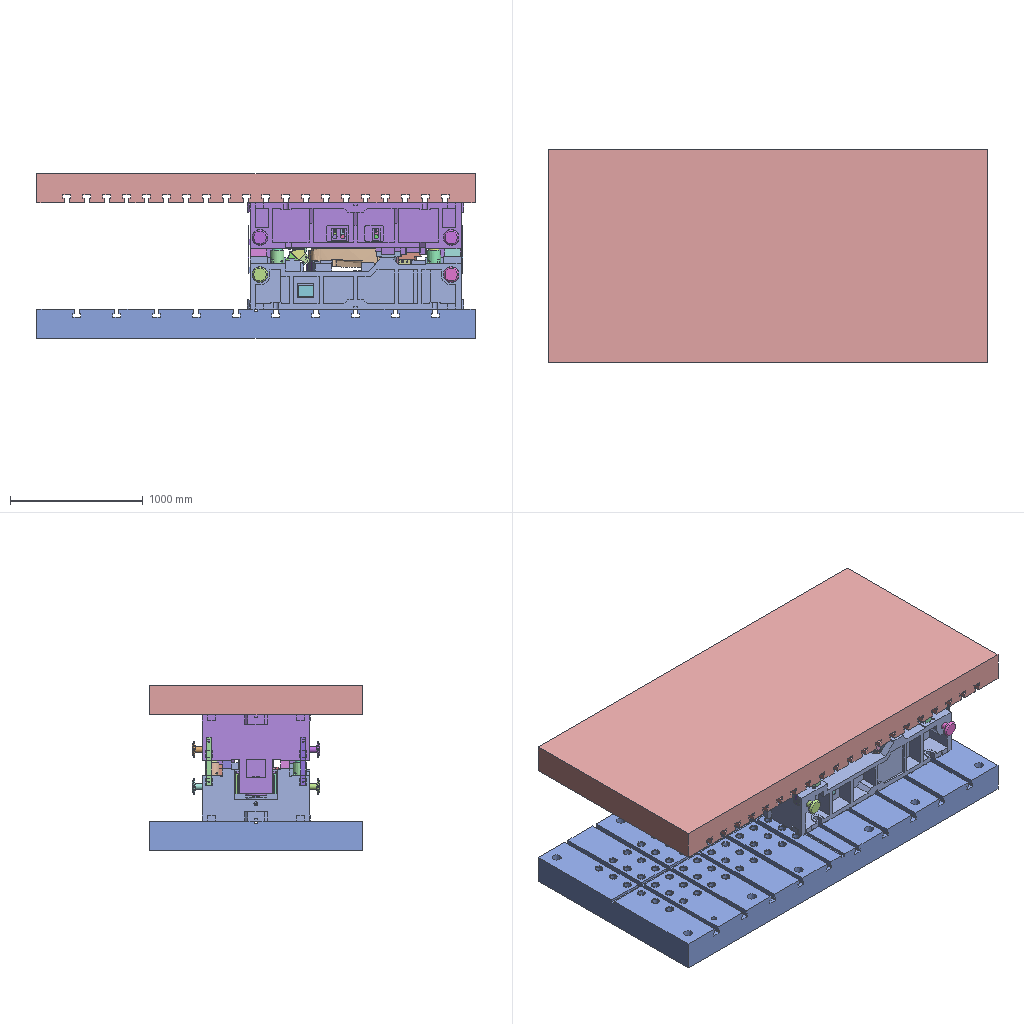Assembly | NX | 112 different items | 112 placed | box 3300 x 1600 x 1240 mm
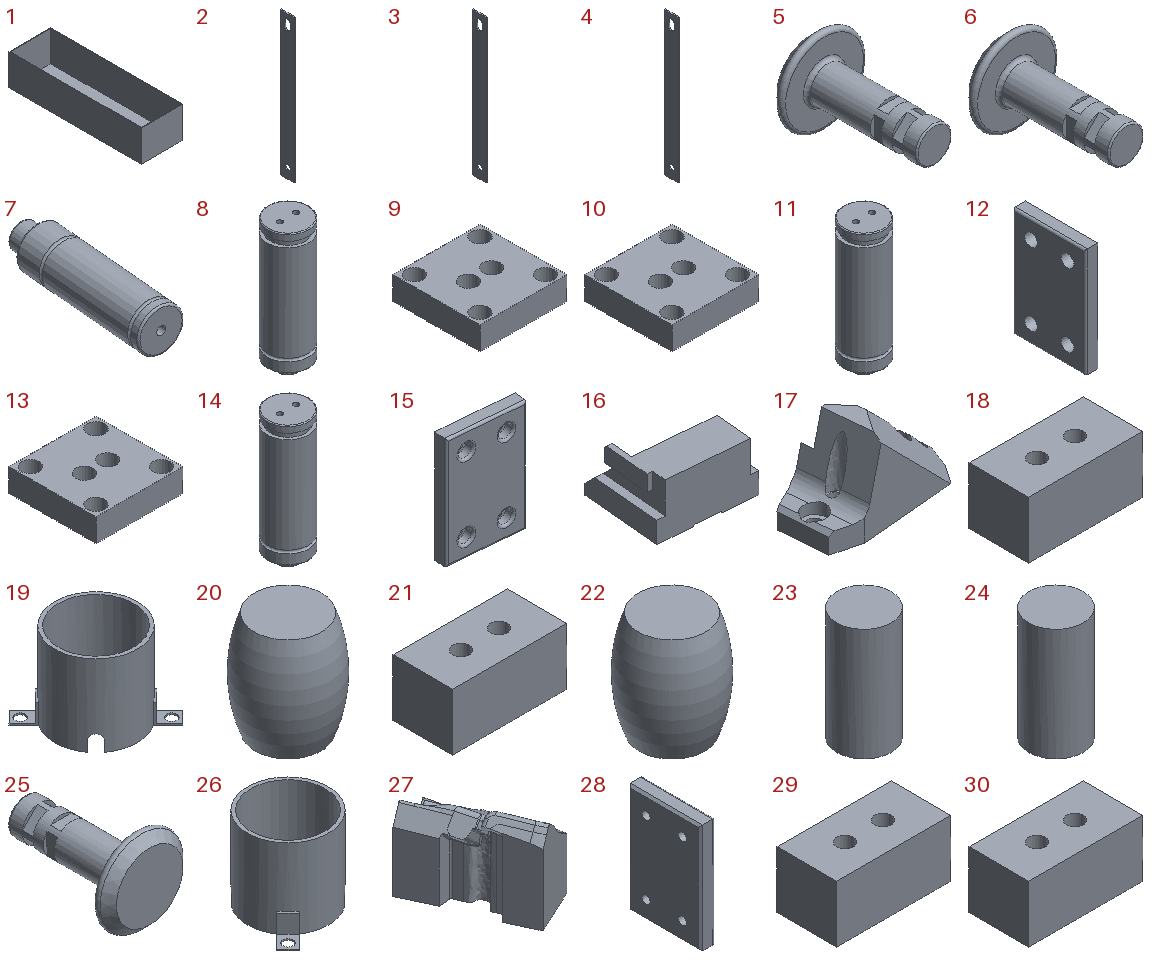Parts list (item | quantity | size | volume | features):
1 | x1 | 120 x 380 x 90 mm | 265792 mm3 | features solid 2
2 | x1 | 3 x 35 x 360 mm | 36435 mm3 | features solid 2
3 | x1 | 3 x 35 x 360 mm | 36435 mm3 | features solid 2
4 | x1 | 3 x 35 x 360 mm | 36435 mm3 | features solid 2
5 | x1 | 120 x 175 x 120 mm | 487590 mm3 | features solid 2
6 | x1 | 120 x 175 x 120 mm | 487590 mm3 | features solid 2
7 | x1 | 31.524 x 91.23 x 24.9 mm | 40004 mm3 | features 1 2
8 | x1 | 50.2 x 50.2 x 160 mm | 293536 mm3 | features 1 2
9 | x1 | 75 x 75 x 20 mm | 96135 mm3 | features 1 2
10 | x1 | 75 x 75 x 20 mm | 96135 mm3 | features 1 2
11 | x1 | 50.2 x 50.2 x 160 mm | 293536 mm3 | features 1 2
12 | x1 | 20 x 100 x 150 mm | 282244 mm3 | features solid 2
13 | x1 | 75 x 75 x 20 mm | 96135 mm3 | features 1 2
14 | x1 | 50.2 x 50.2 x 160 mm | 293536 mm3 | features 1 2
15 | x1 | 100.851 x 28.128 x 150 mm | 281787 mm3 | features MAIN_BODY 2
16 | x1 | 192.388 x 165.117 x 100 mm | 1948955 mm3 | features MAIN_BODY 2
17 | x1 | 107.293 x 58.165 x 63 mm | 136956 mm3 | features solid 2
18 | x1 | 120 x 63 x 60 mm | 430203 mm3 | features solid 2
19 | x1 | 121.34 x 121.34 x 100 mm | 129830 mm3 | features solid 2
20 | x1 | 91.2 x 91.2 x 110 mm | 619751 mm3 | features solid 2
21 | x1 | 120 x 63 x 60 mm | 430203 mm3 | features solid 2
22 | x1 | 91.2 x 91.2 x 110 mm | 619751 mm3 | features solid 2
23 | x1 | 63 x 63 x 140 mm | 407253 mm3 | features solid 2
24 | x1 | 63 x 63 x 140 mm | 407253 mm3 | features solid 2
25 | x1 | 120 x 175 x 120 mm | 487590 mm3 | features solid 2
26 | x1 | 121.34 x 121.34 x 100 mm | 129830 mm3 | features solid 2
27 | x1 | 94.32 x 126.222 x 83.766 mm | 330590 mm3 | features solid 2
28 | x1 | 20 x 100 x 150 mm | 282244 mm3 | features solid 2
29 | x1 | 120 x 63 x 60 mm | 430203 mm3 | features solid 2
30 | x1 | 120 x 63 x 60 mm | 430203 mm3 | features solid 2
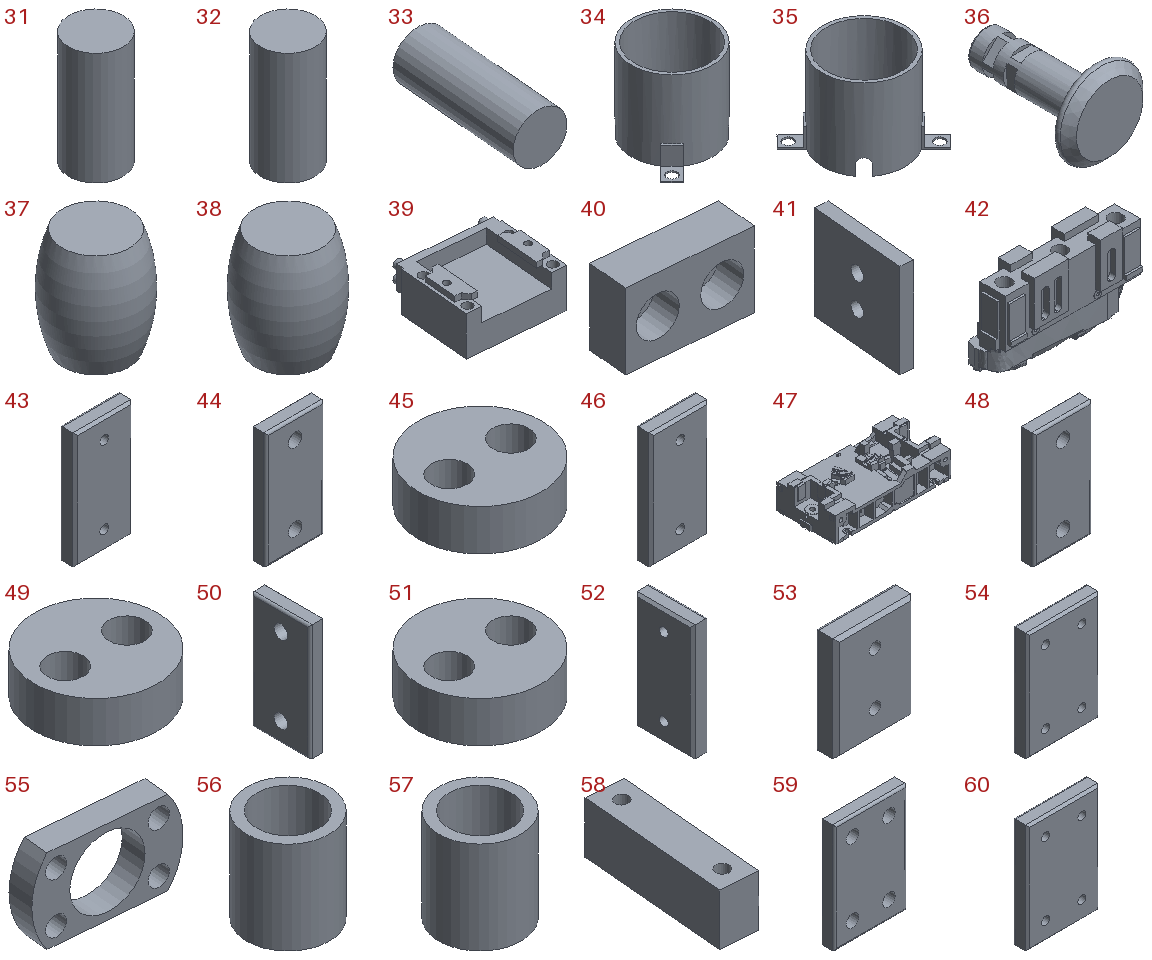31 | x1 | 63 x 63 x 140 mm | 407253 mm3 | features solid 2
32 | x1 | 63 x 63 x 140 mm | 407253 mm3 | features solid 2
33 | x1 | 18.429 x 41.155 x 15 mm | 7069 mm3 | features solid 2
34 | x1 | 121.34 x 121.34 x 100 mm | 129830 mm3 | features solid 2
35 | x1 | 121.34 x 121.34 x 100 mm | 129830 mm3 | features solid 2
36 | x1 | 120 x 175 x 120 mm | 487590 mm3 | features solid 2
37 | x1 | 91.2 x 91.2 x 110 mm | 619751 mm3 | features solid 2
38 | x1 | 91.2 x 91.2 x 110 mm | 619751 mm3 | features solid 2
39 | x1 | 276.442 x 256.978 x 125 mm | 4551984 mm3 | features solid 2
40 | x1 | 61.515 x 25.153 x 38 mm | 35211 mm3 | features solid 2
41 | x1 | 16.499 x 75.586 x 75 mm | 53488 mm3 | features solid 2
42 | x1 | 692.554 x 180 x 425.876 mm | 27420201 mm3 | features solid 2
43 | x1 | 75 x 20 x 150 mm | 214859 mm3 | features solid 2
44 | x1 | 75 x 20 x 150 mm | 214859 mm3 | features solid 2
45 | x1 | 60 x 60 x 20 mm | 48467 mm3 | features solid 2
46 | x1 | 75 x 20 x 150 mm | 214859 mm3 | features solid 2
47 | x1 | 1630 x 815 x 440 mm | 191809441 mm3 | features solid 2
48 | x1 | 75 x 20 x 150 mm | 214859 mm3 | features solid 2
49 | x1 | 60 x 60 x 20 mm | 48467 mm3 | features solid 2
50 | x1 | 20 x 75 x 150 mm | 214859 mm3 | features solid 2
51 | x1 | 60 x 60 x 20 mm | 48467 mm3 | features solid 2
52 | x1 | 20 x 75 x 150 mm | 214859 mm3 | features solid 2
53 | x1 | 75 x 20 x 100 mm | 140502 mm3 | features solid 2
54 | x1 | 100 x 20 x 150 mm | 282244 mm3 | features solid 2
55 | x1 | 50.594 x 13.324 x 30 mm | 6871 mm3 | features solid 2
56 | x1 | 80 x 80 x 90 mm | 197920 mm3 | features solid 2
57 | x1 | 80 x 80 x 90 mm | 197920 mm3 | features solid 2
58 | x1 | 67.241 x 203.597 x 70 mm | 664374 mm3 | features solid 2
59 | x1 | 100 x 20 x 150 mm | 282244 mm3 | features solid 2
60 | x1 | 100 x 20 x 150 mm | 282244 mm3 | features solid 2
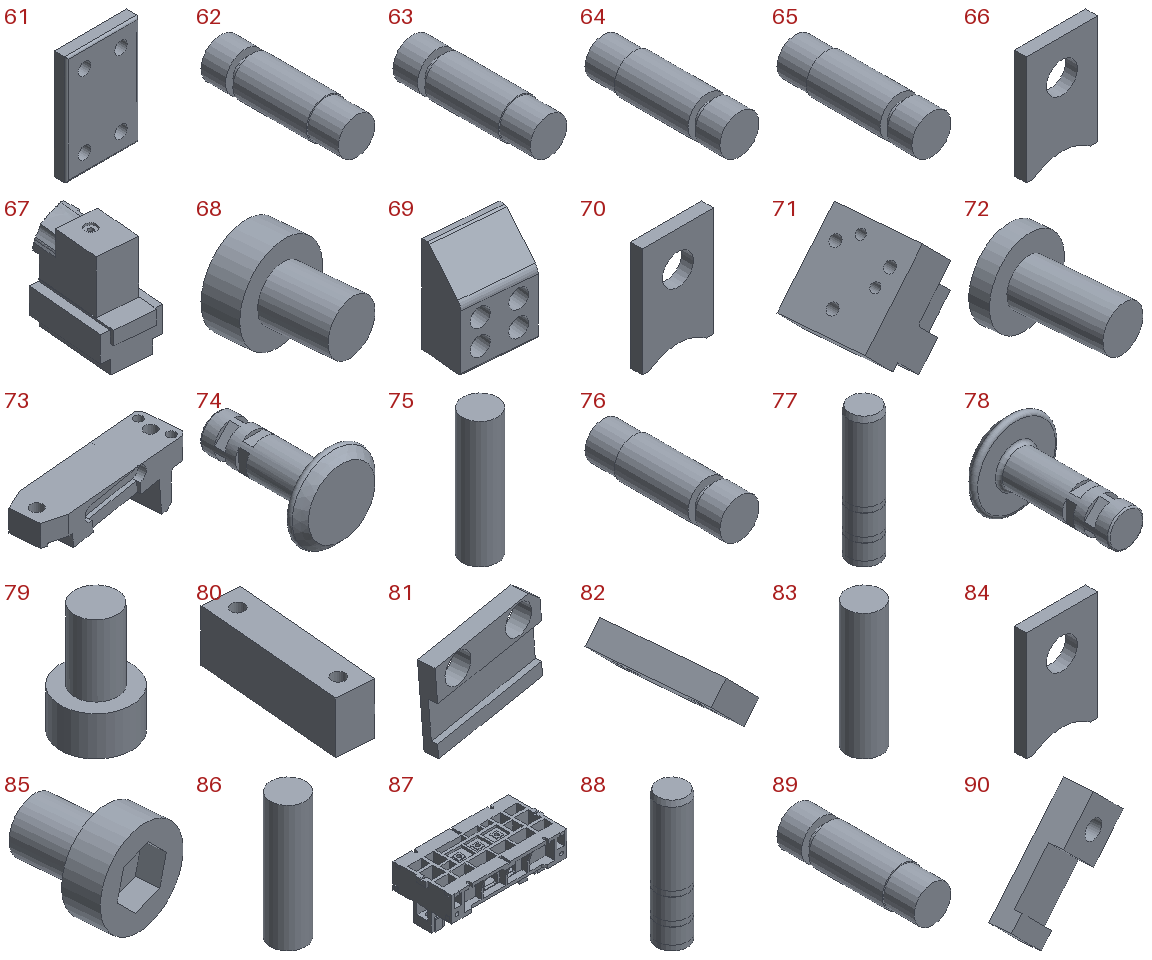61 | x1 | 100 x 20 x 150 mm | 282244 mm3 | features solid 2
62 | x1 | 32 x 111 x 32 mm | 83896 mm3 | features solid 2
63 | x1 | 32 x 111 x 32 mm | 83896 mm3 | features solid 2
64 | x1 | 32 x 111 x 32 mm | 83896 mm3 | features solid 2
65 | x1 | 32 x 111 x 32 mm | 83896 mm3 | features solid 2
66 | x1 | 30 x 5 x 46 mm | 5909 mm3 | features solid 2
67 | x1 | 164.868 x 261.973 x 240 mm | 4872960 mm3 | features solid 2
68 | x1 | 14.426 x 16.398 x 14 mm | 1177 mm3 | features solid 2
69 | x1 | 104.849 x 68.487 x 135 mm | 601030 mm3 | features solid 2
70 | x1 | 30 x 5 x 46 mm | 5909 mm3 | features solid 2
71 | x1 | 91.254 x 60.337 x 86.158 mm | 141612 mm3 | features solid 2
72 | x1 | 13.212 x 17.806 x 13 mm | 871.309 mm3 | features solid 2
73 | x1 | 177.637 x 64.44 x 64.002 mm | 246023 mm3 | features solid 2
74 | x1 | 120 x 175 x 120 mm | 487590 mm3 | features solid 2
75 | x1 | 25 x 25 x 90 mm | 44179 mm3 | features solid 2
76 | x1 | 32 x 111 x 32 mm | 83896 mm3 | features solid 2
77 | x1 | 60 x 60 x 250 mm | 701604 mm3 | features solid 2
78 | x1 | 120 x 175 x 120 mm | 487590 mm3 | features solid 2
79 | x1 | 10.013 x 10.001 x 15.519 mm | 621.654 mm3 | features solid 2
80 | x1 | 67.241 x 203.597 x 70 mm | 664374 mm3 | features solid 2
81 | x1 | 63.975 x 14.011 x 48.539 mm | 13253 mm3 | features solid 2
82 | x1 | 26.899 x 51.782 x 22.627 mm | 9966 mm3 | features solid 2
83 | x1 | 25 x 25 x 90 mm | 44179 mm3 | features solid 2
84 | x1 | 30 x 5 x 46 mm | 5909 mm3 | features solid 2
85 | x1 | 14.426 x 16.398 x 14 mm | 1177 mm3 | features solid 2
86 | x1 | 25 x 25 x 90 mm | 44179 mm3 | features solid 2
87 | x1 | 1630 x 815 x 605 mm | 209531072 mm3 | features solid 2
88 | x1 | 60 x 60 x 250 mm | 701604 mm3 | features solid 2
89 | x1 | 32 x 111 x 32 mm | 83896 mm3 | features solid 2
90 | x1 | 50.355 x 14.419 x 49.497 mm | 7701 mm3 | features solid 2
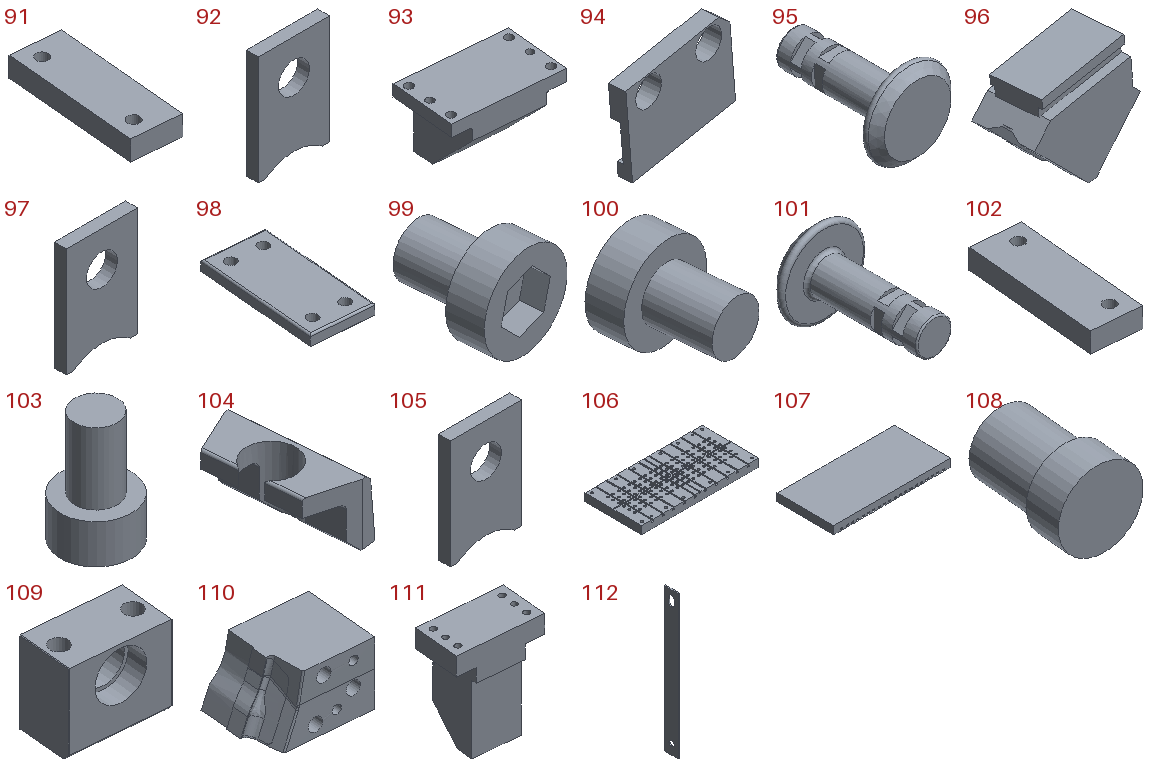91 | x1 | 89.157 x 205.514 x 30 mm | 416732 mm3 | features solid 2
92 | x1 | 30 x 5 x 46 mm | 5909 mm3 | features solid 2
93 | x1 | 241.327 x 159.513 x 160 mm | 2643101 mm3 | features solid 2
94 | x1 | 64.105 x 13.806 x 48.539 mm | 13253 mm3 | features solid 2
95 | x1 | 120 x 175 x 120 mm | 487590 mm3 | features solid 2
96 | x1 | 107.729 x 60.831 x 91.402 mm | 279477 mm3 | features solid 2
97 | x1 | 30 x 5 x 46 mm | 5909 mm3 | features solid 2
98 | x1 | 117.051 x 207.955 x 20 mm | 381601 mm3 | features solid 2
99 | x1 | 14.426 x 16.398 x 14 mm | 1177 mm3 | features solid 2
100 | x1 | 14.426 x 16.398 x 14 mm | 1177 mm3 | features solid 2
101 | x1 | 120 x 175 x 120 mm | 487590 mm3 | features solid 2
102 | x1 | 89.157 x 205.514 x 30 mm | 416732 mm3 | features solid 2
103 | x1 | 10.013 x 10.001 x 15.519 mm | 621.654 mm3 | features solid 2
104 | x1 | 28.396 x 52.31 x 25 mm | 12914 mm3 | features solid 2
105 | x1 | 30 x 5 x 46 mm | 5909 mm3 | features solid 2
106 | x1 | 3300 x 1600 x 220 mm | 1059682394 mm3 | features solid 2
107 | x1 | 3300 x 1600 x 220 mm | 1071834762 mm3 | features solid 2
108 | x1 | 34.182 x 47.443 x 33 mm | 30025 mm3 | features solid 2
109 | x1 | 73.133 x 45.862 x 60 mm | 119047 mm3 | features solid 2
110 | x1 | 133.236 x 104.262 x 80 mm | 713678 mm3 | features solid 2
111 | x1 | 188.031 x 116.802 x 220 mm | 2209901 mm3 | features solid 2
112 | x1 | 3 x 35 x 360 mm | 36435 mm3 | features solid 2